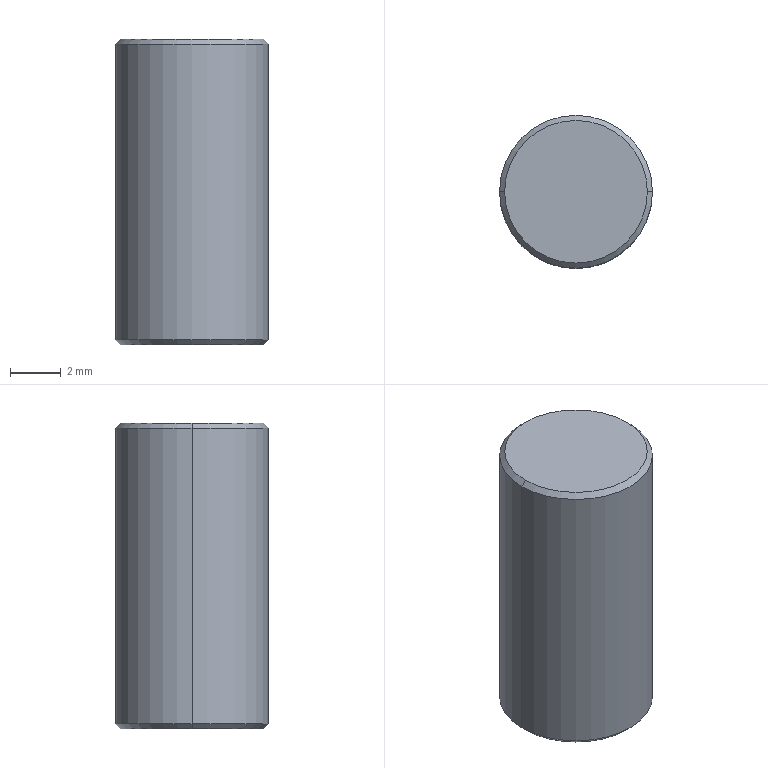Part | STEP file | straight dowel pin 6x12 (g tolerance) | 1 solid | 8 faces | box 6 x 6 x 12 mm | volume 338.555 mm3 | cone 4 | cylinder 2 | plane 2 | commonest cylinder face diameters 6 x2
STEP:
#1=CARTESIAN_POINT('',(0.,0.,0.));
#2=DIRECTION('',(0.,0.,1.));
#3=DIRECTION('',(1.,0.,0.));
#4=AXIS2_PLACEMENT_3D('',#1,#2,#3);
#5=CARTESIAN_POINT('',(-2.8,0.,-12.));
#6=VERTEX_POINT('',#5);
#7=CARTESIAN_POINT('',(2.8,0.,-12.));
#8=VERTEX_POINT('',#7);
#9=CARTESIAN_POINT('',(0.,0.,-12.));
#10=DIRECTION('',(0.,0.,-1.));
#11=DIRECTION('',(-1.,0.,0.));
#12=AXIS2_PLACEMENT_3D('',#9,#10,#11);
#13=CIRCLE('',#12,2.8);
#14=CARTESIAN_POINT('',(0.,0.,-11.8));
#15=DIRECTION('',(0.,0.,1.));
#16=DIRECTION('',(1.,0.,0.));
#17=AXIS2_PLACEMENT_3D('',#14,#15,#16);
#18=CONICAL_SURFACE('',#17,3.,0.7854);
#19=CARTESIAN_POINT('',(3.142,-0.2));
#20=DIRECTION('',(-1.,0.));
#21=VECTOR('',#20,1.);
#22=LINE('',#19,#21);
#23=(GEOMETRIC_REPRESENTATION_CONTEXT(2)PARAMETRIC_REPRESENTATION_CONTEXT()REPRESENTATION_CONTEXT('',''));
#24=DEFINITIONAL_REPRESENTATION('',(#22),#23);
#25=PCURVE('',#18,#24);
#26=CARTESIAN_POINT('',(0.,0.,-12.));
#27=DIRECTION('',(0.,0.,-1.));
#28=DIRECTION('',(-1.,0.,0.));
#29=AXIS2_PLACEMENT_3D('',#26,#27,#28);
#30=PLANE('',#29);
#31=CARTESIAN_POINT('',(0.,0.));
#32=DIRECTION('',(1.,0.));
#33=AXIS2_PLACEMENT_2D('',#31,#32);
#34=CIRCLE('',#33,2.8);
#35=(GEOMETRIC_REPRESENTATION_CONTEXT(2)PARAMETRIC_REPRESENTATION_CONTEXT()REPRESENTATION_CONTEXT('',''));
#36=DEFINITIONAL_REPRESENTATION('',(#34),#35);
#37=PCURVE('',#30,#36);
#38=SURFACE_CURVE('',#13,(#25,#37),.PCURVE_S1.);
#39=EDGE_CURVE('',#6,#8,#38,.T.);
#40=ORIENTED_EDGE('',*,*,#39,.F.);
#41=CARTESIAN_POINT('',(-3.,0.,-11.8));
#42=VERTEX_POINT('',#41);
#43=CARTESIAN_POINT('',(-3.,0.,-11.8));
#44=DIRECTION('',(-0.7071,0.,0.7071));
#45=VECTOR('',#44,1.);
#46=LINE('',#43,#45);
#47=CARTESIAN_POINT('',(3.142,0.));
#48=DIRECTION('',(0.,1.));
#49=VECTOR('',#48,1.);
#50=LINE('',#47,#49);
#51=(GEOMETRIC_REPRESENTATION_CONTEXT(2)PARAMETRIC_REPRESENTATION_CONTEXT()REPRESENTATION_CONTEXT('',''));
#52=DEFINITIONAL_REPRESENTATION('',(#50),#51);
#53=PCURVE('',#18,#52);
#54=CARTESIAN_POINT('',(0.,0.,-11.8));
#55=DIRECTION('',(0.,0.,1.));
#56=DIRECTION('',(1.,0.,0.));
#57=AXIS2_PLACEMENT_3D('',#54,#55,#56);
#58=CONICAL_SURFACE('',#57,3.,0.7854);
#59=CARTESIAN_POINT('',(3.142,0.));
#60=DIRECTION('',(0.,1.));
#61=VECTOR('',#60,1.);
#62=LINE('',#59,#61);
#63=(GEOMETRIC_REPRESENTATION_CONTEXT(2)PARAMETRIC_REPRESENTATION_CONTEXT()REPRESENTATION_CONTEXT('',''));
#64=DEFINITIONAL_REPRESENTATION('',(#62),#63);
#65=PCURVE('',#58,#64);
#66=SURFACE_CURVE('',#46,(#53,#65),.PCURVE_S1.);
#67=EDGE_CURVE('',#6,#42,#66,.T.);
#68=ORIENTED_EDGE('',*,*,#67,.T.);
#69=CARTESIAN_POINT('',(3.,0.,-11.8));
#70=VERTEX_POINT('',#69);
#71=CARTESIAN_POINT('',(0.,0.,-11.8));
#72=DIRECTION('',(0.,0.,1.));
#73=DIRECTION('',(-1.,0.,0.));
#74=AXIS2_PLACEMENT_3D('',#71,#72,#73);
#75=CIRCLE('',#74,3.);
#76=CARTESIAN_POINT('',(-3.142,0.));
#77=DIRECTION('',(1.,0.));
#78=VECTOR('',#77,1.);
#79=LINE('',#76,#78);
#80=(GEOMETRIC_REPRESENTATION_CONTEXT(2)PARAMETRIC_REPRESENTATION_CONTEXT()REPRESENTATION_CONTEXT('',''));
#81=DEFINITIONAL_REPRESENTATION('',(#79),#80);
#82=PCURVE('',#18,#81);
#83=CARTESIAN_POINT('',(0.,0.,0.));
#84=DIRECTION('',(0.,0.,1.));
#85=DIRECTION('',(1.,0.,0.));
#86=AXIS2_PLACEMENT_3D('',#83,#84,#85);
#87=CYLINDRICAL_SURFACE('',#86,3.);
#88=CARTESIAN_POINT('',(-3.142,-11.8));
#89=DIRECTION('',(1.,0.));
#90=VECTOR('',#89,1.);
#91=LINE('',#88,#90);
#92=(GEOMETRIC_REPRESENTATION_CONTEXT(2)PARAMETRIC_REPRESENTATION_CONTEXT()REPRESENTATION_CONTEXT('',''));
#93=DEFINITIONAL_REPRESENTATION('',(#91),#92);
#94=PCURVE('',#87,#93);
#95=SURFACE_CURVE('',#75,(#82,#94),.PCURVE_S1.);
#96=EDGE_CURVE('',#70,#42,#95,.T.);
#97=ORIENTED_EDGE('',*,*,#96,.F.);
#98=CARTESIAN_POINT('',(3.,0.,-11.8));
#99=DIRECTION('',(0.7071,0.,0.7071));
#100=VECTOR('',#99,1.);
#101=LINE('',#98,#100);
#102=CARTESIAN_POINT('',(0.,0.));
#103=DIRECTION('',(0.,1.));
#104=VECTOR('',#103,1.);
#105=LINE('',#102,#104);
#106=(GEOMETRIC_REPRESENTATION_CONTEXT(2)PARAMETRIC_REPRESENTATION_CONTEXT()REPRESENTATION_CONTEXT('',''));
#107=DEFINITIONAL_REPRESENTATION('',(#105),#106);
#108=PCURVE('',#18,#107);
#109=CARTESIAN_POINT('',(6.283,0.));
#110=DIRECTION('',(0.,1.));
#111=VECTOR('',#110,1.);
#112=LINE('',#109,#111);
#113=(GEOMETRIC_REPRESENTATION_CONTEXT(2)PARAMETRIC_REPRESENTATION_CONTEXT()REPRESENTATION_CONTEXT('',''));
#114=DEFINITIONAL_REPRESENTATION('',(#112),#113);
#115=PCURVE('',#58,#114);
#116=SURFACE_CURVE('',#101,(#108,#115),.PCURVE_S1.);
#117=EDGE_CURVE('',#8,#70,#116,.T.);
#118=ORIENTED_EDGE('',*,*,#117,.F.);
#119=EDGE_LOOP('',(#40,#68,#97,#118));
#120=FACE_BOUND('',#119,.T.);
#121=ADVANCED_FACE('',(#120),#18,.T.);
#122=CARTESIAN_POINT('',(2.8,0.,0.));
#123=VERTEX_POINT('',#122);
#124=CARTESIAN_POINT('',(-2.8,0.,0.));
#125=VERTEX_POINT('',#124);
#126=CARTESIAN_POINT('',(0.,0.,0.));
#127=DIRECTION('',(0.,0.,1.));
#128=DIRECTION('',(1.,0.,0.));
#129=AXIS2_PLACEMENT_3D('',#126,#127,#128);
#130=CIRCLE('',#129,2.8);
#131=CARTESIAN_POINT('',(0.,0.,0.));
#132=DIRECTION('',(0.,0.,-1.));
#133=DIRECTION('',(-1.,0.,0.));
#134=AXIS2_PLACEMENT_3D('',#131,#132,#133);
#135=CONICAL_SURFACE('',#134,2.8,0.7854);
#136=CARTESIAN_POINT('',(3.142,0.));
#137=DIRECTION('',(-1.,0.));
#138=VECTOR('',#137,1.);
#139=LINE('',#136,#138);
#140=(GEOMETRIC_REPRESENTATION_CONTEXT(2)PARAMETRIC_REPRESENTATION_CONTEXT()REPRESENTATION_CONTEXT('',''));
#141=DEFINITIONAL_REPRESENTATION('',(#139),#140);
#142=PCURVE('',#135,#141);
#143=CARTESIAN_POINT('',(0.,0.,0.));
#144=DIRECTION('',(0.,0.,1.));
#145=DIRECTION('',(1.,0.,0.));
#146=AXIS2_PLACEMENT_3D('',#143,#144,#145);
#147=PLANE('',#146);
#148=CARTESIAN_POINT('',(0.,0.));
#149=DIRECTION('',(1.,0.));
#150=AXIS2_PLACEMENT_2D('',#148,#149);
#151=CIRCLE('',#150,2.8);
#152=(GEOMETRIC_REPRESENTATION_CONTEXT(2)PARAMETRIC_REPRESENTATION_CONTEXT()REPRESENTATION_CONTEXT('',''));
#153=DEFINITIONAL_REPRESENTATION('',(#151),#152);
#154=PCURVE('',#147,#153);
#155=SURFACE_CURVE('',#130,(#142,#154),.PCURVE_S1.);
#156=EDGE_CURVE('',#123,#125,#155,.T.);
#157=ORIENTED_EDGE('',*,*,#156,.F.);
#158=CARTESIAN_POINT('',(3.,0.,-0.2));
#159=VERTEX_POINT('',#158);
#160=CARTESIAN_POINT('',(2.8,0.,0.));
#161=DIRECTION('',(0.7071,0.,-0.7071));
#162=VECTOR('',#161,1.);
#163=LINE('',#160,#162);
#164=CARTESIAN_POINT('',(3.142,0.));
#165=DIRECTION('',(0.,1.));
#166=VECTOR('',#165,1.);
#167=LINE('',#164,#166);
#168=(GEOMETRIC_REPRESENTATION_CONTEXT(2)PARAMETRIC_REPRESENTATION_CONTEXT()REPRESENTATION_CONTEXT('',''));
#169=DEFINITIONAL_REPRESENTATION('',(#167),#168);
#170=PCURVE('',#135,#169);
#171=CARTESIAN_POINT('',(0.,0.,0.));
#172=DIRECTION('',(0.,0.,-1.));
#173=DIRECTION('',(-1.,0.,0.));
#174=AXIS2_PLACEMENT_3D('',#171,#172,#173);
#175=CONICAL_SURFACE('',#174,2.8,0.7854);
#176=CARTESIAN_POINT('',(3.142,0.));
#177=DIRECTION('',(0.,1.));
#178=VECTOR('',#177,1.);
#179=LINE('',#176,#178);
#180=(GEOMETRIC_REPRESENTATION_CONTEXT(2)PARAMETRIC_REPRESENTATION_CONTEXT()REPRESENTATION_CONTEXT('',''));
#181=DEFINITIONAL_REPRESENTATION('',(#179),#180);
#182=PCURVE('',#175,#181);
#183=SURFACE_CURVE('',#163,(#170,#182),.PCURVE_S1.);
#184=EDGE_CURVE('',#123,#159,#183,.T.);
#185=ORIENTED_EDGE('',*,*,#184,.T.);
#186=CARTESIAN_POINT('',(-3.,0.,-0.2));
#187=VERTEX_POINT('',#186);
#188=CARTESIAN_POINT('',(0.,0.,-0.2));
#189=DIRECTION('',(0.,0.,-1.));
#190=DIRECTION('',(1.,0.,0.));
#191=AXIS2_PLACEMENT_3D('',#188,#189,#190);
#192=CIRCLE('',#191,3.);
#193=CARTESIAN_POINT('',(-3.142,0.2));
#194=DIRECTION('',(1.,0.));
#195=VECTOR('',#194,1.);
#196=LINE('',#193,#195);
#197=(GEOMETRIC_REPRESENTATION_CONTEXT(2)PARAMETRIC_REPRESENTATION_CONTEXT()REPRESENTATION_CONTEXT('',''));
#198=DEFINITIONAL_REPRESENTATION('',(#196),#197);
#199=PCURVE('',#135,#198);
#200=CARTESIAN_POINT('',(6.283,-0.2));
#201=DIRECTION('',(-1.,0.));
#202=VECTOR('',#201,1.);
#203=LINE('',#200,#202);
#204=(GEOMETRIC_REPRESENTATION_CONTEXT(2)PARAMETRIC_REPRESENTATION_CONTEXT()REPRESENTATION_CONTEXT('',''));
#205=DEFINITIONAL_REPRESENTATION('',(#203),#204);
#206=PCURVE('',#87,#205);
#207=SURFACE_CURVE('',#192,(#199,#206),.PCURVE_S1.);
#208=EDGE_CURVE('',#187,#159,#207,.T.);
#209=ORIENTED_EDGE('',*,*,#208,.F.);
#210=CARTESIAN_POINT('',(-2.8,0.,0.));
#211=DIRECTION('',(-0.7071,0.,-0.7071));
#212=VECTOR('',#211,1.);
#213=LINE('',#210,#212);
#214=CARTESIAN_POINT('',(0.,0.));
#215=DIRECTION('',(0.,1.));
#216=VECTOR('',#215,1.);
#217=LINE('',#214,#216);
#218=(GEOMETRIC_REPRESENTATION_CONTEXT(2)PARAMETRIC_REPRESENTATION_CONTEXT()REPRESENTATION_CONTEXT('',''));
#219=DEFINITIONAL_REPRESENTATION('',(#217),#218);
#220=PCURVE('',#135,#219);
#221=CARTESIAN_POINT('',(6.283,0.));
#222=DIRECTION('',(0.,1.));
#223=VECTOR('',#222,1.);
#224=LINE('',#221,#223);
#225=(GEOMETRIC_REPRESENTATION_CONTEXT(2)PARAMETRIC_REPRESENTATION_CONTEXT()REPRESENTATION_CONTEXT('',''));
#226=DEFINITIONAL_REPRESENTATION('',(#224),#225);
#227=PCURVE('',#175,#226);
#228=SURFACE_CURVE('',#213,(#220,#227),.PCURVE_S1.);
#229=EDGE_CURVE('',#125,#187,#228,.T.);
#230=ORIENTED_EDGE('',*,*,#229,.F.);
#231=EDGE_LOOP('',(#157,#185,#209,#230));
#232=FACE_BOUND('',#231,.T.);
#233=ADVANCED_FACE('',(#232),#135,.T.);
#234=ORIENTED_EDGE('',*,*,#96,.T.);
#235=CARTESIAN_POINT('',(-3.,0.,0.));
#236=DIRECTION('',(0.,0.,1.));
#237=VECTOR('',#236,1.);
#238=LINE('',#235,#237);
#239=CARTESIAN_POINT('',(3.142,0.));
#240=DIRECTION('',(0.,1.));
#241=VECTOR('',#240,1.);
#242=LINE('',#239,#241);
#243=(GEOMETRIC_REPRESENTATION_CONTEXT(2)PARAMETRIC_REPRESENTATION_CONTEXT()REPRESENTATION_CONTEXT('',''));
#244=DEFINITIONAL_REPRESENTATION('',(#242),#243);
#245=PCURVE('',#87,#244);
#246=CARTESIAN_POINT('',(0.,0.,0.));
#247=DIRECTION('',(0.,0.,1.));
#248=DIRECTION('',(1.,0.,0.));
#249=AXIS2_PLACEMENT_3D('',#246,#247,#248);
#250=CYLINDRICAL_SURFACE('',#249,3.);
#251=CARTESIAN_POINT('',(3.142,0.));
#252=DIRECTION('',(0.,1.));
#253=VECTOR('',#252,1.);
#254=LINE('',#251,#253);
#255=(GEOMETRIC_REPRESENTATION_CONTEXT(2)PARAMETRIC_REPRESENTATION_CONTEXT()REPRESENTATION_CONTEXT('',''));
#256=DEFINITIONAL_REPRESENTATION('',(#254),#255);
#257=PCURVE('',#250,#256);
#258=SURFACE_CURVE('',#238,(#245,#257),.PCURVE_S1.);
#259=EDGE_CURVE('',#42,#187,#258,.T.);
#260=ORIENTED_EDGE('',*,*,#259,.T.);
#261=ORIENTED_EDGE('',*,*,#208,.T.);
#262=CARTESIAN_POINT('',(3.,0.,0.));
#263=DIRECTION('',(0.,0.,1.));
#264=VECTOR('',#263,1.);
#265=LINE('',#262,#264);
#266=CARTESIAN_POINT('',(0.,0.));
#267=DIRECTION('',(0.,1.));
#268=VECTOR('',#267,1.);
#269=LINE('',#266,#268);
#270=(GEOMETRIC_REPRESENTATION_CONTEXT(2)PARAMETRIC_REPRESENTATION_CONTEXT()REPRESENTATION_CONTEXT('',''));
#271=DEFINITIONAL_REPRESENTATION('',(#269),#270);
#272=PCURVE('',#87,#271);
#273=CARTESIAN_POINT('',(6.283,0.));
#274=DIRECTION('',(0.,1.));
#275=VECTOR('',#274,1.);
#276=LINE('',#273,#275);
#277=(GEOMETRIC_REPRESENTATION_CONTEXT(2)PARAMETRIC_REPRESENTATION_CONTEXT()REPRESENTATION_CONTEXT('',''));
#278=DEFINITIONAL_REPRESENTATION('',(#276),#277);
#279=PCURVE('',#250,#278);
#280=SURFACE_CURVE('',#265,(#272,#279),.PCURVE_S1.);
#281=EDGE_CURVE('',#70,#159,#280,.T.);
#282=ORIENTED_EDGE('',*,*,#281,.F.);
#283=EDGE_LOOP('',(#234,#260,#261,#282));
#284=FACE_BOUND('',#283,.T.);
#285=ADVANCED_FACE('',(#284),#87,.T.);
#286=CARTESIAN_POINT('',(0.,0.,-12.));
#287=DIRECTION('',(0.,0.,-1.));
#288=DIRECTION('',(-1.,0.,0.));
#289=AXIS2_PLACEMENT_3D('',#286,#287,#288);
#290=CIRCLE('',#289,2.8);
#291=CARTESIAN_POINT('',(0.,0.));
#292=DIRECTION('',(1.,0.));
#293=AXIS2_PLACEMENT_2D('',#291,#292);
#294=CIRCLE('',#293,2.8);
#295=(GEOMETRIC_REPRESENTATION_CONTEXT(2)PARAMETRIC_REPRESENTATION_CONTEXT()REPRESENTATION_CONTEXT('',''));
#296=DEFINITIONAL_REPRESENTATION('',(#294),#295);
#297=PCURVE('',#30,#296);
#298=CARTESIAN_POINT('',(9.425,-0.2));
#299=DIRECTION('',(-1.,0.));
#300=VECTOR('',#299,1.);
#301=LINE('',#298,#300);
#302=(GEOMETRIC_REPRESENTATION_CONTEXT(2)PARAMETRIC_REPRESENTATION_CONTEXT()REPRESENTATION_CONTEXT('',''));
#303=DEFINITIONAL_REPRESENTATION('',(#301),#302);
#304=PCURVE('',#58,#303);
#305=SURFACE_CURVE('',#290,(#297,#304),.PCURVE_S1.);
#306=EDGE_CURVE('',#8,#6,#305,.T.);
#307=ORIENTED_EDGE('',*,*,#306,.T.);
#308=ORIENTED_EDGE('',*,*,#39,.T.);
#309=EDGE_LOOP('',(#307,#308));
#310=FACE_BOUND('',#309,.T.);
#311=ADVANCED_FACE('',(#310),#30,.T.);
#312=ORIENTED_EDGE('',*,*,#259,.F.);
#313=CARTESIAN_POINT('',(0.,0.,-11.8));
#314=DIRECTION('',(0.,0.,1.));
#315=DIRECTION('',(-1.,0.,0.));
#316=AXIS2_PLACEMENT_3D('',#313,#314,#315);
#317=CIRCLE('',#316,3.);
#318=CARTESIAN_POINT('',(3.142,-11.8));
#319=DIRECTION('',(1.,0.));
#320=VECTOR('',#319,1.);
#321=LINE('',#318,#320);
#322=(GEOMETRIC_REPRESENTATION_CONTEXT(2)PARAMETRIC_REPRESENTATION_CONTEXT()REPRESENTATION_CONTEXT('',''));
#323=DEFINITIONAL_REPRESENTATION('',(#321),#322);
#324=PCURVE('',#250,#323);
#325=CARTESIAN_POINT('',(3.142,0.));
#326=DIRECTION('',(1.,0.));
#327=VECTOR('',#326,1.);
#328=LINE('',#325,#327);
#329=(GEOMETRIC_REPRESENTATION_CONTEXT(2)PARAMETRIC_REPRESENTATION_CONTEXT()REPRESENTATION_CONTEXT('',''));
#330=DEFINITIONAL_REPRESENTATION('',(#328),#329);
#331=PCURVE('',#58,#330);
#332=SURFACE_CURVE('',#317,(#324,#331),.PCURVE_S1.);
#333=EDGE_CURVE('',#42,#70,#332,.T.);
#334=ORIENTED_EDGE('',*,*,#333,.T.);
#335=ORIENTED_EDGE('',*,*,#281,.T.);
#336=CARTESIAN_POINT('',(0.,0.,-0.2));
#337=DIRECTION('',(0.,0.,-1.));
#338=DIRECTION('',(1.,0.,0.));
#339=AXIS2_PLACEMENT_3D('',#336,#337,#338);
#340=CIRCLE('',#339,3.);
#341=CARTESIAN_POINT('',(6.283,-0.2));
#342=DIRECTION('',(-1.,0.));
#343=VECTOR('',#342,1.);
#344=LINE('',#341,#343);
#345=(GEOMETRIC_REPRESENTATION_CONTEXT(2)PARAMETRIC_REPRESENTATION_CONTEXT()REPRESENTATION_CONTEXT('',''));
#346=DEFINITIONAL_REPRESENTATION('',(#344),#345);
#347=PCURVE('',#250,#346);
#348=CARTESIAN_POINT('',(3.142,0.2));
#349=DIRECTION('',(1.,0.));
#350=VECTOR('',#349,1.);
#351=LINE('',#348,#350);
#352=(GEOMETRIC_REPRESENTATION_CONTEXT(2)PARAMETRIC_REPRESENTATION_CONTEXT()REPRESENTATION_CONTEXT('',''));
#353=DEFINITIONAL_REPRESENTATION('',(#351),#352);
#354=PCURVE('',#175,#353);
#355=SURFACE_CURVE('',#340,(#347,#354),.PCURVE_S1.);
#356=EDGE_CURVE('',#159,#187,#355,.T.);
#357=ORIENTED_EDGE('',*,*,#356,.T.);
#358=EDGE_LOOP('',(#312,#334,#335,#357));
#359=FACE_BOUND('',#358,.T.);
#360=ADVANCED_FACE('',(#359),#250,.T.);
#361=CARTESIAN_POINT('',(0.,0.,0.));
#362=DIRECTION('',(0.,0.,1.));
#363=DIRECTION('',(1.,0.,0.));
#364=AXIS2_PLACEMENT_3D('',#361,#362,#363);
#365=CIRCLE('',#364,2.8);
#366=CARTESIAN_POINT('',(0.,0.));
#367=DIRECTION('',(1.,0.));
#368=AXIS2_PLACEMENT_2D('',#366,#367);
#369=CIRCLE('',#368,2.8);
#370=(GEOMETRIC_REPRESENTATION_CONTEXT(2)PARAMETRIC_REPRESENTATION_CONTEXT()REPRESENTATION_CONTEXT('',''));
#371=DEFINITIONAL_REPRESENTATION('',(#369),#370);
#372=PCURVE('',#147,#371);
#373=CARTESIAN_POINT('',(9.425,0.));
#374=DIRECTION('',(-1.,0.));
#375=VECTOR('',#374,1.);
#376=LINE('',#373,#375);
#377=(GEOMETRIC_REPRESENTATION_CONTEXT(2)PARAMETRIC_REPRESENTATION_CONTEXT()REPRESENTATION_CONTEXT('',''));
#378=DEFINITIONAL_REPRESENTATION('',(#376),#377);
#379=PCURVE('',#175,#378);
#380=SURFACE_CURVE('',#365,(#372,#379),.PCURVE_S1.);
#381=EDGE_CURVE('',#125,#123,#380,.T.);
#382=ORIENTED_EDGE('',*,*,#381,.T.);
#383=ORIENTED_EDGE('',*,*,#156,.T.);
#384=EDGE_LOOP('',(#382,#383));
#385=FACE_BOUND('',#384,.T.);
#386=ADVANCED_FACE('',(#385),#147,.T.);
#387=ORIENTED_EDGE('',*,*,#184,.F.);
#388=ORIENTED_EDGE('',*,*,#381,.F.);
#389=ORIENTED_EDGE('',*,*,#229,.T.);
#390=ORIENTED_EDGE('',*,*,#356,.F.);
#391=EDGE_LOOP('',(#387,#388,#389,#390));
#392=FACE_BOUND('',#391,.T.);
#393=ADVANCED_FACE('',(#392),#175,.T.);
#394=ORIENTED_EDGE('',*,*,#67,.F.);
#395=ORIENTED_EDGE('',*,*,#306,.F.);
#396=ORIENTED_EDGE('',*,*,#117,.T.);
#397=ORIENTED_EDGE('',*,*,#333,.F.);
#398=EDGE_LOOP('',(#394,#395,#396,#397));
#399=FACE_BOUND('',#398,.T.);
#400=ADVANCED_FACE('',(#399),#58,.T.);
#401=CLOSED_SHELL('',(#121,#233,#285,#311,#360,#386,#393,#400));
#402=MANIFOLD_SOLID_BREP('',#401);
#403=(LENGTH_UNIT()NAMED_UNIT(*)SI_UNIT(.MILLI.,.METRE.));
#404=UNCERTAINTY_MEASURE_WITH_UNIT(LENGTH_MEASURE(0.0000001),#403,'','');
#405=(NAMED_UNIT(*)PLANE_ANGLE_UNIT()SI_UNIT($,.RADIAN.));
#406=(NAMED_UNIT(*)SI_UNIT($,.STERADIAN.)SOLID_ANGLE_UNIT());
#407=(GEOMETRIC_REPRESENTATION_CONTEXT(3)GLOBAL_UNCERTAINTY_ASSIGNED_CONTEXT((#404))GLOBAL_UNIT_ASSIGNED_CONTEXT((#403,#405,#406))REPRESENTATION_CONTEXT('',''));
#408=ADVANCED_BREP_SHAPE_REPRESENTATION('',(#4,#402),#407);